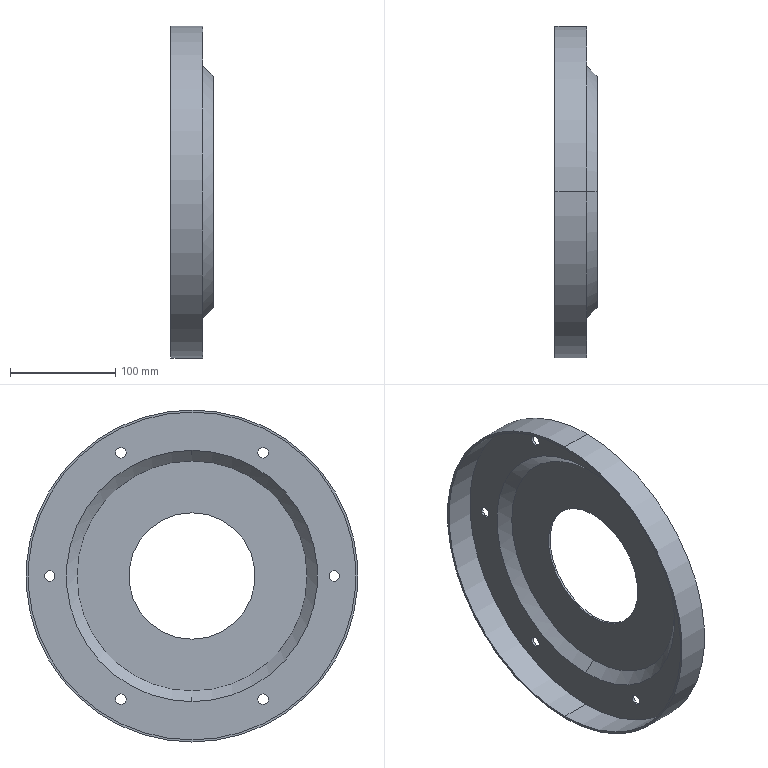Part | SolidWorks | features ICE 2, Revolution 1, Shell 1 | 1 solid | 27 faces | box 40 x 315 x 315 mm | volume 193331 mm3 | cylinder 18 | plane 5 | cone 4 | commonest cylinder face diameters 10 x12 120 x2 311 x2 315 x2
STEP:
#1=CARTESIAN_POINT('',(28.,135.,-5.));
#2=VERTEX_POINT('',#1);
#3=CARTESIAN_POINT('',(28.,135.,5.));
#4=VERTEX_POINT('',#3);
#5=CARTESIAN_POINT('',(28.,135.,0.));
#6=DIRECTION('',(-1.,0.,0.));
#7=DIRECTION('',(0.,0.,1.));
#8=AXIS2_PLACEMENT_3D('',#5,#6,#7);
#9=CIRCLE('',#8,5.);
#10=EDGE_CURVE('',#2,#4,#9,.T.);
#11=ORIENTED_EDGE('',*,*,#10,.T.);
#12=CARTESIAN_POINT('',(30.,135.,5.));
#13=VERTEX_POINT('',#12);
#14=CARTESIAN_POINT('',(-20.,135.,5.));
#15=DIRECTION('',(1.,0.,0.));
#16=VECTOR('',#15,1000.);
#17=LINE('',#14,#16);
#18=EDGE_CURVE('',#4,#13,#17,.T.);
#19=ORIENTED_EDGE('',*,*,#18,.T.);
#20=CARTESIAN_POINT('',(30.,135.,-5.));
#21=VERTEX_POINT('',#20);
#22=CARTESIAN_POINT('',(30.,135.,0.));
#23=DIRECTION('',(1.,0.,0.));
#24=DIRECTION('',(0.,0.,-1.));
#25=AXIS2_PLACEMENT_3D('',#22,#23,#24);
#26=CIRCLE('',#25,5.);
#27=EDGE_CURVE('',#13,#21,#26,.T.);
#28=ORIENTED_EDGE('',*,*,#27,.T.);
#29=CARTESIAN_POINT('',(-20.,135.,-5.));
#30=DIRECTION('',(1.,0.,0.));
#31=VECTOR('',#30,1000.);
#32=LINE('',#29,#31);
#33=EDGE_CURVE('',#2,#21,#32,.T.);
#34=ORIENTED_EDGE('',*,*,#33,.F.);
#35=EDGE_LOOP('',(#11,#19,#28,#34));
#36=FACE_OUTER_BOUND('',#35,.T.);
#37=CARTESIAN_POINT('',(-20.,135.,0.));
#38=DIRECTION('',(1.,0.,0.));
#39=DIRECTION('',(0.,0.,-1.));
#40=AXIS2_PLACEMENT_3D('',#37,#38,#39);
#41=CYLINDRICAL_SURFACE('',#40,5.);
#42=ADVANCED_FACE('',(#36),#41,.F.);
#43=CARTESIAN_POINT('',(28.,67.5,111.913));
#44=VERTEX_POINT('',#43);
#45=CARTESIAN_POINT('',(28.,67.5,121.913));
#46=VERTEX_POINT('',#45);
#47=CARTESIAN_POINT('',(28.,67.5,116.913));
#48=DIRECTION('',(-1.,0.,0.));
#49=DIRECTION('',(0.,0.,1.));
#50=AXIS2_PLACEMENT_3D('',#47,#48,#49);
#51=CIRCLE('',#50,5.);
#52=EDGE_CURVE('',#44,#46,#51,.T.);
#53=ORIENTED_EDGE('',*,*,#52,.T.);
#54=CARTESIAN_POINT('',(30.,67.5,121.913));
#55=VERTEX_POINT('',#54);
#56=CARTESIAN_POINT('',(-20.,67.5,121.913));
#57=DIRECTION('',(1.,0.,0.));
#58=VECTOR('',#57,1000.);
#59=LINE('',#56,#58);
#60=EDGE_CURVE('',#46,#55,#59,.T.);
#61=ORIENTED_EDGE('',*,*,#60,.T.);
#62=CARTESIAN_POINT('',(30.,67.5,111.913));
#63=VERTEX_POINT('',#62);
#64=CARTESIAN_POINT('',(30.,67.5,116.913));
#65=DIRECTION('',(1.,0.,0.));
#66=DIRECTION('',(0.,0.,-1.));
#67=AXIS2_PLACEMENT_3D('',#64,#65,#66);
#68=CIRCLE('',#67,5.);
#69=EDGE_CURVE('',#55,#63,#68,.T.);
#70=ORIENTED_EDGE('',*,*,#69,.T.);
#71=CARTESIAN_POINT('',(-20.,67.5,111.913));
#72=DIRECTION('',(1.,0.,0.));
#73=VECTOR('',#72,1000.);
#74=LINE('',#71,#73);
#75=EDGE_CURVE('',#44,#63,#74,.T.);
#76=ORIENTED_EDGE('',*,*,#75,.F.);
#77=EDGE_LOOP('',(#53,#61,#70,#76));
#78=FACE_OUTER_BOUND('',#77,.T.);
#79=CARTESIAN_POINT('',(-20.,67.5,116.913));
#80=DIRECTION('',(1.,0.,0.));
#81=DIRECTION('',(0.,0.,-1.));
#82=AXIS2_PLACEMENT_3D('',#79,#80,#81);
#83=CYLINDRICAL_SURFACE('',#82,5.);
#84=ADVANCED_FACE('',(#78),#83,.F.);
#85=CARTESIAN_POINT('',(28.,-67.5,111.913));
#86=VERTEX_POINT('',#85);
#87=CARTESIAN_POINT('',(28.,-67.5,121.913));
#88=VERTEX_POINT('',#87);
#89=CARTESIAN_POINT('',(28.,-67.5,116.913));
#90=DIRECTION('',(-1.,0.,0.));
#91=DIRECTION('',(0.,0.,1.));
#92=AXIS2_PLACEMENT_3D('',#89,#90,#91);
#93=CIRCLE('',#92,5.);
#94=EDGE_CURVE('',#86,#88,#93,.T.);
#95=ORIENTED_EDGE('',*,*,#94,.T.);
#96=CARTESIAN_POINT('',(30.,-67.5,121.913));
#97=VERTEX_POINT('',#96);
#98=CARTESIAN_POINT('',(-20.,-67.5,121.913));
#99=DIRECTION('',(1.,0.,0.));
#100=VECTOR('',#99,1000.);
#101=LINE('',#98,#100);
#102=EDGE_CURVE('',#88,#97,#101,.T.);
#103=ORIENTED_EDGE('',*,*,#102,.T.);
#104=CARTESIAN_POINT('',(30.,-67.5,111.913));
#105=VERTEX_POINT('',#104);
#106=CARTESIAN_POINT('',(30.,-67.5,116.913));
#107=DIRECTION('',(1.,0.,0.));
#108=DIRECTION('',(0.,0.,-1.));
#109=AXIS2_PLACEMENT_3D('',#106,#107,#108);
#110=CIRCLE('',#109,5.);
#111=EDGE_CURVE('',#97,#105,#110,.T.);
#112=ORIENTED_EDGE('',*,*,#111,.T.);
#113=CARTESIAN_POINT('',(-20.,-67.5,111.913));
#114=DIRECTION('',(1.,0.,0.));
#115=VECTOR('',#114,1000.);
#116=LINE('',#113,#115);
#117=EDGE_CURVE('',#86,#105,#116,.T.);
#118=ORIENTED_EDGE('',*,*,#117,.F.);
#119=EDGE_LOOP('',(#95,#103,#112,#118));
#120=FACE_OUTER_BOUND('',#119,.T.);
#121=CARTESIAN_POINT('',(-20.,-67.5,116.913));
#122=DIRECTION('',(1.,0.,0.));
#123=DIRECTION('',(0.,0.,-1.));
#124=AXIS2_PLACEMENT_3D('',#121,#122,#123);
#125=CYLINDRICAL_SURFACE('',#124,5.);
#126=ADVANCED_FACE('',(#120),#125,.F.);
#127=CARTESIAN_POINT('',(28.,-135.,-5.));
#128=VERTEX_POINT('',#127);
#129=CARTESIAN_POINT('',(28.,-135.,5.));
#130=VERTEX_POINT('',#129);
#131=CARTESIAN_POINT('',(28.,-135.,0.));
#132=DIRECTION('',(-1.,0.,0.));
#133=DIRECTION('',(0.,0.,1.));
#134=AXIS2_PLACEMENT_3D('',#131,#132,#133);
#135=CIRCLE('',#134,5.);
#136=EDGE_CURVE('',#128,#130,#135,.T.);
#137=ORIENTED_EDGE('',*,*,#136,.T.);
#138=CARTESIAN_POINT('',(30.,-135.,5.));
#139=VERTEX_POINT('',#138);
#140=CARTESIAN_POINT('',(-20.,-135.,5.));
#141=DIRECTION('',(1.,0.,0.));
#142=VECTOR('',#141,1000.);
#143=LINE('',#140,#142);
#144=EDGE_CURVE('',#130,#139,#143,.T.);
#145=ORIENTED_EDGE('',*,*,#144,.T.);
#146=CARTESIAN_POINT('',(30.,-135.,-5.));
#147=VERTEX_POINT('',#146);
#148=CARTESIAN_POINT('',(30.,-135.,0.));
#149=DIRECTION('',(1.,0.,0.));
#150=DIRECTION('',(0.,0.,-1.));
#151=AXIS2_PLACEMENT_3D('',#148,#149,#150);
#152=CIRCLE('',#151,5.);
#153=EDGE_CURVE('',#139,#147,#152,.T.);
#154=ORIENTED_EDGE('',*,*,#153,.T.);
#155=CARTESIAN_POINT('',(-20.,-135.,-5.));
#156=DIRECTION('',(1.,0.,0.));
#157=VECTOR('',#156,1000.);
#158=LINE('',#155,#157);
#159=EDGE_CURVE('',#128,#147,#158,.T.);
#160=ORIENTED_EDGE('',*,*,#159,.F.);
#161=EDGE_LOOP('',(#137,#145,#154,#160));
#162=FACE_OUTER_BOUND('',#161,.T.);
#163=CARTESIAN_POINT('',(-20.,-135.,0.));
#164=DIRECTION('',(1.,0.,0.));
#165=DIRECTION('',(0.,0.,-1.));
#166=AXIS2_PLACEMENT_3D('',#163,#164,#165);
#167=CYLINDRICAL_SURFACE('',#166,5.);
#168=ADVANCED_FACE('',(#162),#167,.F.);
#169=CARTESIAN_POINT('',(28.,-67.5,-121.913));
#170=VERTEX_POINT('',#169);
#171=CARTESIAN_POINT('',(28.,-67.5,-111.913));
#172=VERTEX_POINT('',#171);
#173=CARTESIAN_POINT('',(28.,-67.5,-116.913));
#174=DIRECTION('',(-1.,0.,0.));
#175=DIRECTION('',(0.,0.,1.));
#176=AXIS2_PLACEMENT_3D('',#173,#174,#175);
#177=CIRCLE('',#176,5.);
#178=EDGE_CURVE('',#170,#172,#177,.T.);
#179=ORIENTED_EDGE('',*,*,#178,.T.);
#180=CARTESIAN_POINT('',(30.,-67.5,-111.913));
#181=VERTEX_POINT('',#180);
#182=CARTESIAN_POINT('',(-20.,-67.5,-111.913));
#183=DIRECTION('',(1.,0.,0.));
#184=VECTOR('',#183,1000.);
#185=LINE('',#182,#184);
#186=EDGE_CURVE('',#172,#181,#185,.T.);
#187=ORIENTED_EDGE('',*,*,#186,.T.);
#188=CARTESIAN_POINT('',(30.,-67.5,-121.913));
#189=VERTEX_POINT('',#188);
#190=CARTESIAN_POINT('',(30.,-67.5,-116.913));
#191=DIRECTION('',(1.,0.,0.));
#192=DIRECTION('',(0.,0.,-1.));
#193=AXIS2_PLACEMENT_3D('',#190,#191,#192);
#194=CIRCLE('',#193,5.);
#195=EDGE_CURVE('',#181,#189,#194,.T.);
#196=ORIENTED_EDGE('',*,*,#195,.T.);
#197=CARTESIAN_POINT('',(-20.,-67.5,-121.913));
#198=DIRECTION('',(1.,0.,0.));
#199=VECTOR('',#198,1000.);
#200=LINE('',#197,#199);
#201=EDGE_CURVE('',#170,#189,#200,.T.);
#202=ORIENTED_EDGE('',*,*,#201,.F.);
#203=EDGE_LOOP('',(#179,#187,#196,#202));
#204=FACE_OUTER_BOUND('',#203,.T.);
#205=CARTESIAN_POINT('',(-20.,-67.5,-116.913));
#206=DIRECTION('',(1.,0.,0.));
#207=DIRECTION('',(0.,0.,-1.));
#208=AXIS2_PLACEMENT_3D('',#205,#206,#207);
#209=CYLINDRICAL_SURFACE('',#208,5.);
#210=ADVANCED_FACE('',(#204),#209,.F.);
#211=CARTESIAN_POINT('',(28.,67.5,-121.913));
#212=VERTEX_POINT('',#211);
#213=CARTESIAN_POINT('',(28.,67.5,-111.913));
#214=VERTEX_POINT('',#213);
#215=CARTESIAN_POINT('',(28.,67.5,-116.913));
#216=DIRECTION('',(-1.,0.,0.));
#217=DIRECTION('',(0.,0.,1.));
#218=AXIS2_PLACEMENT_3D('',#215,#216,#217);
#219=CIRCLE('',#218,5.);
#220=EDGE_CURVE('',#212,#214,#219,.T.);
#221=ORIENTED_EDGE('',*,*,#220,.T.);
#222=CARTESIAN_POINT('',(30.,67.5,-111.913));
#223=VERTEX_POINT('',#222);
#224=CARTESIAN_POINT('',(-20.,67.5,-111.913));
#225=DIRECTION('',(1.,0.,0.));
#226=VECTOR('',#225,1000.);
#227=LINE('',#224,#226);
#228=EDGE_CURVE('',#214,#223,#227,.T.);
#229=ORIENTED_EDGE('',*,*,#228,.T.);
#230=CARTESIAN_POINT('',(30.,67.5,-121.913));
#231=VERTEX_POINT('',#230);
#232=CARTESIAN_POINT('',(30.,67.5,-116.913));
#233=DIRECTION('',(1.,0.,0.));
#234=DIRECTION('',(0.,0.,-1.));
#235=AXIS2_PLACEMENT_3D('',#232,#233,#234);
#236=CIRCLE('',#235,5.);
#237=EDGE_CURVE('',#223,#231,#236,.T.);
#238=ORIENTED_EDGE('',*,*,#237,.T.);
#239=CARTESIAN_POINT('',(-20.,67.5,-121.913));
#240=DIRECTION('',(1.,0.,0.));
#241=VECTOR('',#240,1000.);
#242=LINE('',#239,#241);
#243=EDGE_CURVE('',#212,#231,#242,.T.);
#244=ORIENTED_EDGE('',*,*,#243,.F.);
#245=EDGE_LOOP('',(#221,#229,#238,#244));
#246=FACE_OUTER_BOUND('',#245,.T.);
#247=CARTESIAN_POINT('',(-20.,67.5,-116.913));
#248=DIRECTION('',(1.,0.,0.));
#249=DIRECTION('',(0.,0.,-1.));
#250=AXIS2_PLACEMENT_3D('',#247,#248,#249);
#251=CYLINDRICAL_SURFACE('',#250,5.);
#252=ADVANCED_FACE('',(#246),#251,.F.);
#253=CARTESIAN_POINT('',(38.,0.,-60.));
#254=VERTEX_POINT('',#253);
#255=CARTESIAN_POINT('',(38.,0.,60.));
#256=VERTEX_POINT('',#255);
#257=CARTESIAN_POINT('',(38.,0.,0.));
#258=DIRECTION('',(-1.,0.,0.));
#259=DIRECTION('',(0.,0.,1.));
#260=AXIS2_PLACEMENT_3D('',#257,#258,#259);
#261=CIRCLE('',#260,60.);
#262=EDGE_CURVE('',#254,#256,#261,.T.);
#263=ORIENTED_EDGE('',*,*,#262,.T.);
#264=CARTESIAN_POINT('',(40.,0.,60.));
#265=VERTEX_POINT('',#264);
#266=CARTESIAN_POINT('',(-10.,0.,60.));
#267=DIRECTION('',(1.,0.,0.));
#268=VECTOR('',#267,1000.);
#269=LINE('',#266,#268);
#270=EDGE_CURVE('',#256,#265,#269,.T.);
#271=ORIENTED_EDGE('',*,*,#270,.T.);
#272=CARTESIAN_POINT('',(40.,0.,-60.));
#273=VERTEX_POINT('',#272);
#274=CARTESIAN_POINT('',(40.,0.,0.));
#275=DIRECTION('',(1.,0.,0.));
#276=DIRECTION('',(0.,0.,-1.));
#277=AXIS2_PLACEMENT_3D('',#274,#275,#276);
#278=CIRCLE('',#277,60.);
#279=EDGE_CURVE('',#265,#273,#278,.T.);
#280=ORIENTED_EDGE('',*,*,#279,.T.);
#281=CARTESIAN_POINT('',(-10.,0.,-60.));
#282=DIRECTION('',(1.,0.,0.));
#283=VECTOR('',#282,1000.);
#284=LINE('',#281,#283);
#285=EDGE_CURVE('',#254,#273,#284,.T.);
#286=ORIENTED_EDGE('',*,*,#285,.F.);
#287=EDGE_LOOP('',(#263,#271,#280,#286));
#288=FACE_OUTER_BOUND('',#287,.T.);
#289=CARTESIAN_POINT('',(-10.,0.,0.));
#290=DIRECTION('',(1.,0.,0.));
#291=DIRECTION('',(0.,0.,-1.));
#292=AXIS2_PLACEMENT_3D('',#289,#290,#291);
#293=CYLINDRICAL_SURFACE('',#292,60.);
#294=ADVANCED_FACE('',(#288),#293,.F.);
#295=CARTESIAN_POINT('',(38.,0.,-109.172));
#296=VERTEX_POINT('',#295);
#297=CARTESIAN_POINT('',(38.,0.,109.172));
#298=VERTEX_POINT('',#297);
#299=CARTESIAN_POINT('',(38.,0.,0.));
#300=DIRECTION('',(-1.,0.,0.));
#301=DIRECTION('',(0.,0.,1.));
#302=AXIS2_PLACEMENT_3D('',#299,#300,#301);
#303=CIRCLE('',#302,109.172);
#304=EDGE_CURVE('',#296,#298,#303,.T.);
#305=ORIENTED_EDGE('',*,*,#304,.F.);
#306=CARTESIAN_POINT('',(28.,0.,-119.172));
#307=VERTEX_POINT('',#306);
#308=CARTESIAN_POINT('',(38.586,0.,-108.586));
#309=DIRECTION('',(-0.7071,0.,-0.7071));
#310=VECTOR('',#309,1000.);
#311=LINE('',#308,#310);
#312=EDGE_CURVE('',#296,#307,#311,.T.);
#313=ORIENTED_EDGE('',*,*,#312,.T.);
#314=CARTESIAN_POINT('',(28.,0.,119.172));
#315=VERTEX_POINT('',#314);
#316=CARTESIAN_POINT('',(28.,0.,0.));
#317=DIRECTION('',(-1.,0.,0.));
#318=DIRECTION('',(0.,0.,1.));
#319=AXIS2_PLACEMENT_3D('',#316,#317,#318);
#320=CIRCLE('',#319,119.172);
#321=EDGE_CURVE('',#307,#315,#320,.T.);
#322=ORIENTED_EDGE('',*,*,#321,.T.);
#323=CARTESIAN_POINT('',(38.586,0.,108.586));
#324=DIRECTION('',(-0.7071,0.,0.7071));
#325=VECTOR('',#324,1000.);
#326=LINE('',#323,#325);
#327=EDGE_CURVE('',#298,#315,#326,.T.);
#328=ORIENTED_EDGE('',*,*,#327,.F.);
#329=EDGE_LOOP('',(#305,#313,#322,#328));
#330=FACE_OUTER_BOUND('',#329,.T.);
#331=CARTESIAN_POINT('',(38.586,0.,0.));
#332=DIRECTION('',(-1.,0.,0.));
#333=DIRECTION('',(0.,0.,1.));
#334=AXIS2_PLACEMENT_3D('',#331,#332,#333);
#335=CONICAL_SURFACE('',#334,108.586,0.7854);
#336=ADVANCED_FACE('',(#330),#335,.F.);
#337=CARTESIAN_POINT('',(28.,0.,-155.5));
#338=VERTEX_POINT('',#337);
#339=CARTESIAN_POINT('',(28.,0.,155.5));
#340=VERTEX_POINT('',#339);
#341=CARTESIAN_POINT('',(28.,0.,0.));
#342=DIRECTION('',(-1.,0.,0.));
#343=DIRECTION('',(0.,0.,1.));
#344=AXIS2_PLACEMENT_3D('',#341,#342,#343);
#345=CIRCLE('',#344,155.5);
#346=EDGE_CURVE('',#338,#340,#345,.T.);
#347=ORIENTED_EDGE('',*,*,#346,.F.);
#348=CARTESIAN_POINT('',(0.,0.,-155.5));
#349=VERTEX_POINT('',#348);
#350=CARTESIAN_POINT('',(0.,0.,-155.5));
#351=DIRECTION('',(-1.,0.,0.));
#352=VECTOR('',#351,1000.);
#353=LINE('',#350,#352);
#354=EDGE_CURVE('',#338,#349,#353,.T.);
#355=ORIENTED_EDGE('',*,*,#354,.T.);
#356=CARTESIAN_POINT('',(0.,0.,155.5));
#357=VERTEX_POINT('',#356);
#358=CARTESIAN_POINT('',(0.,0.,0.));
#359=DIRECTION('',(-1.,0.,0.));
#360=DIRECTION('',(0.,0.,-1.));
#361=AXIS2_PLACEMENT_3D('',#358,#359,#360);
#362=CIRCLE('',#361,155.5);
#363=EDGE_CURVE('',#349,#357,#362,.T.);
#364=ORIENTED_EDGE('',*,*,#363,.T.);
#365=CARTESIAN_POINT('',(0.,0.,155.5));
#366=DIRECTION('',(-1.,0.,0.));
#367=VECTOR('',#366,1000.);
#368=LINE('',#365,#367);
#369=EDGE_CURVE('',#340,#357,#368,.T.);
#370=ORIENTED_EDGE('',*,*,#369,.F.);
#371=EDGE_LOOP('',(#347,#355,#364,#370));
#372=FACE_OUTER_BOUND('',#371,.T.);
#373=CARTESIAN_POINT('',(0.,0.,0.));
#374=DIRECTION('',(-1.,0.,0.));
#375=DIRECTION('',(0.,0.,1.));
#376=AXIS2_PLACEMENT_3D('',#373,#374,#375);
#377=CYLINDRICAL_SURFACE('',#376,155.5);
#378=ADVANCED_FACE('',(#372),#377,.F.);
#379=CARTESIAN_POINT('',(40.,0.,110.));
#380=VERTEX_POINT('',#379);
#381=CARTESIAN_POINT('',(40.,0.,-110.));
#382=VERTEX_POINT('',#381);
#383=CARTESIAN_POINT('',(40.,0.,0.));
#384=DIRECTION('',(-1.,0.,0.));
#385=DIRECTION('',(0.,0.,1.));
#386=AXIS2_PLACEMENT_3D('',#383,#384,#385);
#387=CIRCLE('',#386,110.);
#388=EDGE_CURVE('',#380,#382,#387,.T.);
#389=ORIENTED_EDGE('',*,*,#388,.T.);
#390=CARTESIAN_POINT('',(30.,0.,-120.));
#391=VERTEX_POINT('',#390);
#392=CARTESIAN_POINT('',(40.,0.,-110.));
#393=DIRECTION('',(-0.7071,0.,-0.7071));
#394=VECTOR('',#393,1000.);
#395=LINE('',#392,#394);
#396=EDGE_CURVE('',#382,#391,#395,.T.);
#397=ORIENTED_EDGE('',*,*,#396,.T.);
#398=CARTESIAN_POINT('',(30.,0.,120.));
#399=VERTEX_POINT('',#398);
#400=CARTESIAN_POINT('',(30.,0.,0.));
#401=DIRECTION('',(-1.,0.,0.));
#402=DIRECTION('',(0.,0.,1.));
#403=AXIS2_PLACEMENT_3D('',#400,#401,#402);
#404=CIRCLE('',#403,120.);
#405=EDGE_CURVE('',#399,#391,#404,.T.);
#406=ORIENTED_EDGE('',*,*,#405,.F.);
#407=CARTESIAN_POINT('',(40.,0.,110.));
#408=DIRECTION('',(-0.7071,0.,0.7071));
#409=VECTOR('',#408,1000.);
#410=LINE('',#407,#409);
#411=EDGE_CURVE('',#380,#399,#410,.T.);
#412=ORIENTED_EDGE('',*,*,#411,.F.);
#413=EDGE_LOOP('',(#389,#397,#406,#412));
#414=FACE_OUTER_BOUND('',#413,.T.);
#415=CARTESIAN_POINT('',(40.,0.,0.));
#416=DIRECTION('',(-1.,0.,0.));
#417=DIRECTION('',(0.,0.,1.));
#418=AXIS2_PLACEMENT_3D('',#415,#416,#417);
#419=CONICAL_SURFACE('',#418,110.,0.7854);
#420=ADVANCED_FACE('',(#414),#419,.T.);
#421=CARTESIAN_POINT('',(30.,0.,157.5));
#422=VERTEX_POINT('',#421);
#423=CARTESIAN_POINT('',(30.,0.,-157.5));
#424=VERTEX_POINT('',#423);
#425=CARTESIAN_POINT('',(30.,0.,0.));
#426=DIRECTION('',(-1.,0.,0.));
#427=DIRECTION('',(0.,0.,1.));
#428=AXIS2_PLACEMENT_3D('',#425,#426,#427);
#429=CIRCLE('',#428,157.5);
#430=EDGE_CURVE('',#422,#424,#429,.T.);
#431=ORIENTED_EDGE('',*,*,#430,.T.);
#432=CARTESIAN_POINT('',(0.,0.,-157.5));
#433=VERTEX_POINT('',#432);
#434=CARTESIAN_POINT('',(0.,0.,-157.5));
#435=DIRECTION('',(-1.,0.,0.));
#436=VECTOR('',#435,1000.);
#437=LINE('',#434,#436);
#438=EDGE_CURVE('',#424,#433,#437,.T.);
#439=ORIENTED_EDGE('',*,*,#438,.T.);
#440=CARTESIAN_POINT('',(0.,0.,157.5));
#441=VERTEX_POINT('',#440);
#442=CARTESIAN_POINT('',(0.,0.,0.));
#443=DIRECTION('',(-1.,0.,0.));
#444=DIRECTION('',(0.,0.,1.));
#445=AXIS2_PLACEMENT_3D('',#442,#443,#444);
#446=CIRCLE('',#445,157.5);
#447=EDGE_CURVE('',#441,#433,#446,.T.);
#448=ORIENTED_EDGE('',*,*,#447,.F.);
#449=CARTESIAN_POINT('',(0.,0.,157.5));
#450=DIRECTION('',(-1.,0.,0.));
#451=VECTOR('',#450,1000.);
#452=LINE('',#449,#451);
#453=EDGE_CURVE('',#422,#441,#452,.T.);
#454=ORIENTED_EDGE('',*,*,#453,.F.);
#455=EDGE_LOOP('',(#431,#439,#448,#454));
#456=FACE_OUTER_BOUND('',#455,.T.);
#457=CARTESIAN_POINT('',(0.,0.,0.));
#458=DIRECTION('',(-1.,0.,0.));
#459=DIRECTION('',(0.,0.,1.));
#460=AXIS2_PLACEMENT_3D('',#457,#458,#459);
#461=CYLINDRICAL_SURFACE('',#460,157.5);
#462=ADVANCED_FACE('',(#456),#461,.T.);
#463=CARTESIAN_POINT('',(0.,0.,0.));
#464=DIRECTION('',(-1.,0.,0.));
#465=DIRECTION('',(0.,0.,-1.));
#466=AXIS2_PLACEMENT_3D('',#463,#464,#465);
#467=CIRCLE('',#466,155.5);
#468=EDGE_CURVE('',#357,#349,#467,.T.);
#469=ORIENTED_EDGE('',*,*,#468,.F.);
#470=ORIENTED_EDGE('',*,*,#363,.F.);
#471=EDGE_LOOP('',(#469,#470));
#472=FACE_BOUND('',#471,.T.);
#473=ORIENTED_EDGE('',*,*,#447,.T.);
#474=CARTESIAN_POINT('',(0.,0.,0.));
#475=DIRECTION('',(-1.,0.,0.));
#476=DIRECTION('',(0.,0.,1.));
#477=AXIS2_PLACEMENT_3D('',#474,#475,#476);
#478=CIRCLE('',#477,157.5);
#479=EDGE_CURVE('',#433,#441,#478,.T.);
#480=ORIENTED_EDGE('',*,*,#479,.T.);
#481=EDGE_LOOP('',(#473,#480));
#482=FACE_OUTER_BOUND('',#481,.T.);
#483=CARTESIAN_POINT('',(0.,0.,0.));
#484=DIRECTION('',(1.,0.,0.));
#485=DIRECTION('',(0.,0.,-1.));
#486=AXIS2_PLACEMENT_3D('',#483,#484,#485);
#487=PLANE('',#486);
#488=ADVANCED_FACE('',(#472,#482),#487,.F.);
#489=ORIENTED_EDGE('',*,*,#438,.F.);
#490=CARTESIAN_POINT('',(30.,0.,0.));
#491=DIRECTION('',(-1.,0.,0.));
#492=DIRECTION('',(0.,0.,1.));
#493=AXIS2_PLACEMENT_3D('',#490,#491,#492);
#494=CIRCLE('',#493,157.5);
#495=EDGE_CURVE('',#424,#422,#494,.T.);
#496=ORIENTED_EDGE('',*,*,#495,.T.);
#497=ORIENTED_EDGE('',*,*,#453,.T.);
#498=ORIENTED_EDGE('',*,*,#479,.F.);
#499=EDGE_LOOP('',(#489,#496,#497,#498));
#500=FACE_OUTER_BOUND('',#499,.T.);
#501=CARTESIAN_POINT('',(0.,0.,0.));
#502=DIRECTION('',(-1.,0.,0.));
#503=DIRECTION('',(0.,0.,1.));
#504=AXIS2_PLACEMENT_3D('',#501,#502,#503);
#505=CYLINDRICAL_SURFACE('',#504,157.5);
#506=ADVANCED_FACE('',(#500),#505,.T.);
#507=CARTESIAN_POINT('',(30.,135.,0.));
#508=DIRECTION('',(1.,0.,0.));
#509=DIRECTION('',(0.,0.,-1.));
#510=AXIS2_PLACEMENT_3D('',#507,#508,#509);
#511=CIRCLE('',#510,5.);
#512=EDGE_CURVE('',#21,#13,#511,.T.);
#513=ORIENTED_EDGE('',*,*,#512,.F.);
#514=ORIENTED_EDGE('',*,*,#27,.F.);
#515=EDGE_LOOP('',(#513,#514));
#516=FACE_BOUND('',#515,.T.);
#517=CARTESIAN_POINT('',(30.,67.5,116.913));
#518=DIRECTION('',(1.,0.,0.));
#519=DIRECTION('',(0.,0.,-1.));
#520=AXIS2_PLACEMENT_3D('',#517,#518,#519);
#521=CIRCLE('',#520,5.);
#522=EDGE_CURVE('',#63,#55,#521,.T.);
#523=ORIENTED_EDGE('',*,*,#522,.F.);
#524=ORIENTED_EDGE('',*,*,#69,.F.);
#525=EDGE_LOOP('',(#523,#524));
#526=FACE_BOUND('',#525,.T.);
#527=CARTESIAN_POINT('',(30.,-67.5,116.913));
#528=DIRECTION('',(1.,0.,0.));
#529=DIRECTION('',(0.,0.,-1.));
#530=AXIS2_PLACEMENT_3D('',#527,#528,#529);
#531=CIRCLE('',#530,5.);
#532=EDGE_CURVE('',#105,#97,#531,.T.);
#533=ORIENTED_EDGE('',*,*,#532,.F.);
#534=ORIENTED_EDGE('',*,*,#111,.F.);
#535=EDGE_LOOP('',(#533,#534));
#536=FACE_BOUND('',#535,.T.);
#537=CARTESIAN_POINT('',(30.,-135.,0.));
#538=DIRECTION('',(1.,0.,0.));
#539=DIRECTION('',(0.,0.,-1.));
#540=AXIS2_PLACEMENT_3D('',#537,#538,#539);
#541=CIRCLE('',#540,5.);
#542=EDGE_CURVE('',#147,#139,#541,.T.);
#543=ORIENTED_EDGE('',*,*,#542,.F.);
#544=ORIENTED_EDGE('',*,*,#153,.F.);
#545=EDGE_LOOP('',(#543,#544));
#546=FACE_BOUND('',#545,.T.);
#547=CARTESIAN_POINT('',(30.,-67.5,-116.913));
#548=DIRECTION('',(1.,0.,0.));
#549=DIRECTION('',(0.,0.,-1.));
#550=AXIS2_PLACEMENT_3D('',#547,#548,#549);
#551=CIRCLE('',#550,5.);
#552=EDGE_CURVE('',#189,#181,#551,.T.);
#553=ORIENTED_EDGE('',*,*,#552,.F.);
#554=ORIENTED_EDGE('',*,*,#195,.F.);
#555=EDGE_LOOP('',(#553,#554));
#556=FACE_BOUND('',#555,.T.);
#557=CARTESIAN_POINT('',(30.,67.5,-116.913));
#558=DIRECTION('',(1.,0.,0.));
#559=DIRECTION('',(0.,0.,-1.));
#560=AXIS2_PLACEMENT_3D('',#557,#558,#559);
#561=CIRCLE('',#560,5.);
#562=EDGE_CURVE('',#231,#223,#561,.T.);
#563=ORIENTED_EDGE('',*,*,#562,.F.);
#564=ORIENTED_EDGE('',*,*,#237,.F.);
#565=EDGE_LOOP('',(#563,#564));
#566=FACE_BOUND('',#565,.T.);
#567=ORIENTED_EDGE('',*,*,#430,.F.);
#568=ORIENTED_EDGE('',*,*,#495,.F.);
#569=EDGE_LOOP('',(#567,#568));
#570=FACE_OUTER_BOUND('',#569,.T.);
#571=ORIENTED_EDGE('',*,*,#405,.T.);
#572=CARTESIAN_POINT('',(30.,0.,0.));
#573=DIRECTION('',(-1.,0.,0.));
#574=DIRECTION('',(0.,0.,1.));
#575=AXIS2_PLACEMENT_3D('',#572,#573,#574);
#576=CIRCLE('',#575,120.);
#577=EDGE_CURVE('',#391,#399,#576,.T.);
#578=ORIENTED_EDGE('',*,*,#577,.T.);
#579=EDGE_LOOP('',(#571,#578));
#580=FACE_BOUND('',#579,.T.);
#581=CARTESIAN_POINT('',(30.,0.,-157.5));
#582=DIRECTION('',(-1.,0.,0.));
#583=DIRECTION('',(0.,0.,1.));
#584=AXIS2_PLACEMENT_3D('',#581,#582,#583);
#585=PLANE('',#584);
#586=ADVANCED_FACE('',(#516,#526,#536,#546,#556,#566,#570,#580),#585,.F.);
#587=ORIENTED_EDGE('',*,*,#396,.F.);
#588=CARTESIAN_POINT('',(40.,0.,0.));
#589=DIRECTION('',(-1.,0.,0.));
#590=DIRECTION('',(0.,0.,1.));
#591=AXIS2_PLACEMENT_3D('',#588,#589,#590);
#592=CIRCLE('',#591,110.);
#593=EDGE_CURVE('',#382,#380,#592,.T.);
#594=ORIENTED_EDGE('',*,*,#593,.T.);
#595=ORIENTED_EDGE('',*,*,#411,.T.);
#596=ORIENTED_EDGE('',*,*,#577,.F.);
#597=EDGE_LOOP('',(#587,#594,#595,#596));
#598=FACE_OUTER_BOUND('',#597,.T.);
#599=CARTESIAN_POINT('',(40.,0.,0.));
#600=DIRECTION('',(-1.,0.,0.));
#601=DIRECTION('',(0.,0.,1.));
#602=AXIS2_PLACEMENT_3D('',#599,#600,#601);
#603=CONICAL_SURFACE('',#602,110.,0.7854);
#604=ADVANCED_FACE('',(#598),#603,.T.);
#605=CARTESIAN_POINT('',(40.,0.,0.));
#606=DIRECTION('',(1.,0.,0.));
#607=DIRECTION('',(0.,0.,-1.));
#608=AXIS2_PLACEMENT_3D('',#605,#606,#607);
#609=CIRCLE('',#608,60.);
#610=EDGE_CURVE('',#273,#265,#609,.T.);
#611=ORIENTED_EDGE('',*,*,#610,.F.);
#612=ORIENTED_EDGE('',*,*,#279,.F.);
#613=EDGE_LOOP('',(#611,#612));
#614=FACE_BOUND('',#613,.T.);
#615=ORIENTED_EDGE('',*,*,#388,.F.);
#616=ORIENTED_EDGE('',*,*,#593,.F.);
#617=EDGE_LOOP('',(#615,#616));
#618=FACE_OUTER_BOUND('',#617,.T.);
#619=CARTESIAN_POINT('',(40.,0.,-110.));
#620=DIRECTION('',(-1.,0.,0.));
#621=DIRECTION('',(0.,0.,1.));
#622=AXIS2_PLACEMENT_3D('',#619,#620,#621);
#623=PLANE('',#622);
#624=ADVANCED_FACE('',(#614,#618),#623,.F.);
#625=ORIENTED_EDGE('',*,*,#354,.F.);
#626=CARTESIAN_POINT('',(28.,0.,0.));
#627=DIRECTION('',(-1.,0.,0.));
#628=DIRECTION('',(0.,0.,1.));
#629=AXIS2_PLACEMENT_3D('',#626,#627,#628);
#630=CIRCLE('',#629,155.5);
#631=EDGE_CURVE('',#340,#338,#630,.T.);
#632=ORIENTED_EDGE('',*,*,#631,.F.);
#633=ORIENTED_EDGE('',*,*,#369,.T.);
#634=ORIENTED_EDGE('',*,*,#468,.T.);
#635=EDGE_LOOP('',(#625,#632,#633,#634));
#636=FACE_OUTER_BOUND('',#635,.T.);
#637=CARTESIAN_POINT('',(0.,0.,0.));
#638=DIRECTION('',(-1.,0.,0.));
#639=DIRECTION('',(0.,0.,1.));
#640=AXIS2_PLACEMENT_3D('',#637,#638,#639);
#641=CYLINDRICAL_SURFACE('',#640,155.5);
#642=ADVANCED_FACE('',(#636),#641,.F.);
#643=ORIENTED_EDGE('',*,*,#10,.F.);
#644=CARTESIAN_POINT('',(28.,135.,0.));
#645=DIRECTION('',(-1.,0.,0.));
#646=DIRECTION('',(0.,0.,1.));
#647=AXIS2_PLACEMENT_3D('',#644,#645,#646);
#648=CIRCLE('',#647,5.);
#649=EDGE_CURVE('',#4,#2,#648,.T.);
#650=ORIENTED_EDGE('',*,*,#649,.F.);
#651=EDGE_LOOP('',(#643,#650));
#652=FACE_BOUND('',#651,.T.);
#653=ORIENTED_EDGE('',*,*,#52,.F.);
#654=CARTESIAN_POINT('',(28.,67.5,116.913));
#655=DIRECTION('',(-1.,0.,0.));
#656=DIRECTION('',(0.,0.,1.));
#657=AXIS2_PLACEMENT_3D('',#654,#655,#656);
#658=CIRCLE('',#657,5.);
#659=EDGE_CURVE('',#46,#44,#658,.T.);
#660=ORIENTED_EDGE('',*,*,#659,.F.);
#661=EDGE_LOOP('',(#653,#660));
#662=FACE_BOUND('',#661,.T.);
#663=ORIENTED_EDGE('',*,*,#94,.F.);
#664=CARTESIAN_POINT('',(28.,-67.5,116.913));
#665=DIRECTION('',(-1.,0.,0.));
#666=DIRECTION('',(0.,0.,1.));
#667=AXIS2_PLACEMENT_3D('',#664,#665,#666);
#668=CIRCLE('',#667,5.);
#669=EDGE_CURVE('',#88,#86,#668,.T.);
#670=ORIENTED_EDGE('',*,*,#669,.F.);
#671=EDGE_LOOP('',(#663,#670));
#672=FACE_BOUND('',#671,.T.);
#673=ORIENTED_EDGE('',*,*,#136,.F.);
#674=CARTESIAN_POINT('',(28.,-135.,0.));
#675=DIRECTION('',(-1.,0.,0.));
#676=DIRECTION('',(0.,0.,1.));
#677=AXIS2_PLACEMENT_3D('',#674,#675,#676);
#678=CIRCLE('',#677,5.);
#679=EDGE_CURVE('',#130,#128,#678,.T.);
#680=ORIENTED_EDGE('',*,*,#679,.F.);
#681=EDGE_LOOP('',(#673,#680));
#682=FACE_BOUND('',#681,.T.);
#683=ORIENTED_EDGE('',*,*,#178,.F.);
#684=CARTESIAN_POINT('',(28.,-67.5,-116.913));
#685=DIRECTION('',(-1.,0.,0.));
#686=DIRECTION('',(0.,0.,1.));
#687=AXIS2_PLACEMENT_3D('',#684,#685,#686);
#688=CIRCLE('',#687,5.);
#689=EDGE_CURVE('',#172,#170,#688,.T.);
#690=ORIENTED_EDGE('',*,*,#689,.F.);
#691=EDGE_LOOP('',(#683,#690));
#692=FACE_BOUND('',#691,.T.);
#693=ORIENTED_EDGE('',*,*,#220,.F.);
#694=CARTESIAN_POINT('',(28.,67.5,-116.913));
#695=DIRECTION('',(-1.,0.,0.));
#696=DIRECTION('',(0.,0.,1.));
#697=AXIS2_PLACEMENT_3D('',#694,#695,#696);
#698=CIRCLE('',#697,5.);
#699=EDGE_CURVE('',#214,#212,#698,.T.);
#700=ORIENTED_EDGE('',*,*,#699,.F.);
#701=EDGE_LOOP('',(#693,#700));
#702=FACE_BOUND('',#701,.T.);
#703=ORIENTED_EDGE('',*,*,#631,.T.);
#704=ORIENTED_EDGE('',*,*,#346,.T.);
#705=EDGE_LOOP('',(#703,#704));
#706=FACE_OUTER_BOUND('',#705,.T.);
#707=CARTESIAN_POINT('',(28.,0.,0.));
#708=DIRECTION('',(-1.,0.,0.));
#709=DIRECTION('',(0.,0.,1.));
#710=AXIS2_PLACEMENT_3D('',#707,#708,#709);
#711=CIRCLE('',#710,119.172);
#712=EDGE_CURVE('',#315,#307,#711,.T.);
#713=ORIENTED_EDGE('',*,*,#712,.F.);
#714=ORIENTED_EDGE('',*,*,#321,.F.);
#715=EDGE_LOOP('',(#713,#714));
#716=FACE_BOUND('',#715,.T.);
#717=CARTESIAN_POINT('',(28.,0.,-157.5));
#718=DIRECTION('',(-1.,0.,0.));
#719=DIRECTION('',(0.,0.,1.));
#720=AXIS2_PLACEMENT_3D('',#717,#718,#719);
#721=PLANE('',#720);
#722=ADVANCED_FACE('',(#652,#662,#672,#682,#692,#702,#706,#716),#721,.T.);
#723=ORIENTED_EDGE('',*,*,#312,.F.);
#724=CARTESIAN_POINT('',(38.,0.,0.));
#725=DIRECTION('',(-1.,0.,0.));
#726=DIRECTION('',(0.,0.,1.));
#727=AXIS2_PLACEMENT_3D('',#724,#725,#726);
#728=CIRCLE('',#727,109.172);
#729=EDGE_CURVE('',#298,#296,#728,.T.);
#730=ORIENTED_EDGE('',*,*,#729,.F.);
#731=ORIENTED_EDGE('',*,*,#327,.T.);
#732=ORIENTED_EDGE('',*,*,#712,.T.);
#733=EDGE_LOOP('',(#723,#730,#731,#732));
#734=FACE_OUTER_BOUND('',#733,.T.);
#735=CARTESIAN_POINT('',(38.586,0.,0.));
#736=DIRECTION('',(-1.,0.,0.));
#737=DIRECTION('',(0.,0.,1.));
#738=AXIS2_PLACEMENT_3D('',#735,#736,#737);
#739=CONICAL_SURFACE('',#738,108.586,0.7854);
#740=ADVANCED_FACE('',(#734),#739,.F.);
#741=ORIENTED_EDGE('',*,*,#262,.F.);
#742=CARTESIAN_POINT('',(38.,0.,0.));
#743=DIRECTION('',(-1.,0.,0.));
#744=DIRECTION('',(0.,0.,1.));
#745=AXIS2_PLACEMENT_3D('',#742,#743,#744);
#746=CIRCLE('',#745,60.);
#747=EDGE_CURVE('',#256,#254,#746,.T.);
#748=ORIENTED_EDGE('',*,*,#747,.F.);
#749=EDGE_LOOP('',(#741,#748));
#750=FACE_BOUND('',#749,.T.);
#751=ORIENTED_EDGE('',*,*,#729,.T.);
#752=ORIENTED_EDGE('',*,*,#304,.T.);
#753=EDGE_LOOP('',(#751,#752));
#754=FACE_OUTER_BOUND('',#753,.T.);
#755=CARTESIAN_POINT('',(38.,0.,-110.));
#756=DIRECTION('',(-1.,0.,0.));
#757=DIRECTION('',(0.,0.,1.));
#758=AXIS2_PLACEMENT_3D('',#755,#756,#757);
#759=PLANE('',#758);
#760=ADVANCED_FACE('',(#750,#754),#759,.T.);
#761=ORIENTED_EDGE('',*,*,#270,.F.);
#762=ORIENTED_EDGE('',*,*,#747,.T.);
#763=ORIENTED_EDGE('',*,*,#285,.T.);
#764=ORIENTED_EDGE('',*,*,#610,.T.);
#765=EDGE_LOOP('',(#761,#762,#763,#764));
#766=FACE_OUTER_BOUND('',#765,.T.);
#767=CARTESIAN_POINT('',(-10.,0.,0.));
#768=DIRECTION('',(1.,0.,0.));
#769=DIRECTION('',(0.,0.,-1.));
#770=AXIS2_PLACEMENT_3D('',#767,#768,#769);
#771=CYLINDRICAL_SURFACE('',#770,60.);
#772=ADVANCED_FACE('',(#766),#771,.F.);
#773=ORIENTED_EDGE('',*,*,#228,.F.);
#774=ORIENTED_EDGE('',*,*,#699,.T.);
#775=ORIENTED_EDGE('',*,*,#243,.T.);
#776=ORIENTED_EDGE('',*,*,#562,.T.);
#777=EDGE_LOOP('',(#773,#774,#775,#776));
#778=FACE_OUTER_BOUND('',#777,.T.);
#779=CARTESIAN_POINT('',(-20.,67.5,-116.913));
#780=DIRECTION('',(1.,0.,0.));
#781=DIRECTION('',(0.,0.,-1.));
#782=AXIS2_PLACEMENT_3D('',#779,#780,#781);
#783=CYLINDRICAL_SURFACE('',#782,5.);
#784=ADVANCED_FACE('',(#778),#783,.F.);
#785=ORIENTED_EDGE('',*,*,#186,.F.);
#786=ORIENTED_EDGE('',*,*,#689,.T.);
#787=ORIENTED_EDGE('',*,*,#201,.T.);
#788=ORIENTED_EDGE('',*,*,#552,.T.);
#789=EDGE_LOOP('',(#785,#786,#787,#788));
#790=FACE_OUTER_BOUND('',#789,.T.);
#791=CARTESIAN_POINT('',(-20.,-67.5,-116.913));
#792=DIRECTION('',(1.,0.,0.));
#793=DIRECTION('',(0.,0.,-1.));
#794=AXIS2_PLACEMENT_3D('',#791,#792,#793);
#795=CYLINDRICAL_SURFACE('',#794,5.);
#796=ADVANCED_FACE('',(#790),#795,.F.);
#797=ORIENTED_EDGE('',*,*,#144,.F.);
#798=ORIENTED_EDGE('',*,*,#679,.T.);
#799=ORIENTED_EDGE('',*,*,#159,.T.);
#800=ORIENTED_EDGE('',*,*,#542,.T.);
#801=EDGE_LOOP('',(#797,#798,#799,#800));
#802=FACE_OUTER_BOUND('',#801,.T.);
#803=CARTESIAN_POINT('',(-20.,-135.,0.));
#804=DIRECTION('',(1.,0.,0.));
#805=DIRECTION('',(0.,0.,-1.));
#806=AXIS2_PLACEMENT_3D('',#803,#804,#805);
#807=CYLINDRICAL_SURFACE('',#806,5.);
#808=ADVANCED_FACE('',(#802),#807,.F.);
#809=ORIENTED_EDGE('',*,*,#102,.F.);
#810=ORIENTED_EDGE('',*,*,#669,.T.);
#811=ORIENTED_EDGE('',*,*,#117,.T.);
#812=ORIENTED_EDGE('',*,*,#532,.T.);
#813=EDGE_LOOP('',(#809,#810,#811,#812));
#814=FACE_OUTER_BOUND('',#813,.T.);
#815=CARTESIAN_POINT('',(-20.,-67.5,116.913));
#816=DIRECTION('',(1.,0.,0.));
#817=DIRECTION('',(0.,0.,-1.));
#818=AXIS2_PLACEMENT_3D('',#815,#816,#817);
#819=CYLINDRICAL_SURFACE('',#818,5.);
#820=ADVANCED_FACE('',(#814),#819,.F.);
#821=ORIENTED_EDGE('',*,*,#60,.F.);
#822=ORIENTED_EDGE('',*,*,#659,.T.);
#823=ORIENTED_EDGE('',*,*,#75,.T.);
#824=ORIENTED_EDGE('',*,*,#522,.T.);
#825=EDGE_LOOP('',(#821,#822,#823,#824));
#826=FACE_OUTER_BOUND('',#825,.T.);
#827=CARTESIAN_POINT('',(-20.,67.5,116.913));
#828=DIRECTION('',(1.,0.,0.));
#829=DIRECTION('',(0.,0.,-1.));
#830=AXIS2_PLACEMENT_3D('',#827,#828,#829);
#831=CYLINDRICAL_SURFACE('',#830,5.);
#832=ADVANCED_FACE('',(#826),#831,.F.);
#833=ORIENTED_EDGE('',*,*,#18,.F.);
#834=ORIENTED_EDGE('',*,*,#649,.T.);
#835=ORIENTED_EDGE('',*,*,#33,.T.);
#836=ORIENTED_EDGE('',*,*,#512,.T.);
#837=EDGE_LOOP('',(#833,#834,#835,#836));
#838=FACE_OUTER_BOUND('',#837,.T.);
#839=CARTESIAN_POINT('',(-20.,135.,0.));
#840=DIRECTION('',(1.,0.,0.));
#841=DIRECTION('',(0.,0.,-1.));
#842=AXIS2_PLACEMENT_3D('',#839,#840,#841);
#843=CYLINDRICAL_SURFACE('',#842,5.);
#844=ADVANCED_FACE('',(#838),#843,.F.);
#845=CLOSED_SHELL('',(#42,#84,#126,#168,#210,#252,#294,#336,#378,#420,#462,#488,#506,#586,#604,#624,#642,#722,#740,#760,#772,#784,#796,#808,#820,#832,#844));
#846=MANIFOLD_SOLID_BREP('',#845);
#847=CARTESIAN_POINT('',(0.,0.,0.));
#848=DIRECTION('',(0.,0.,1.));
#849=DIRECTION('',(1.,0.,0.));
#850=AXIS2_PLACEMENT_3D('',#847,#848,#849);
#851=(LENGTH_UNIT()NAMED_UNIT(*)SI_UNIT(.MILLI.,.METRE.));
#852=UNCERTAINTY_MEASURE_WITH_UNIT(LENGTH_MEASURE(0.00001),#851,'','');
#853=(NAMED_UNIT(*)PLANE_ANGLE_UNIT()SI_UNIT($,.RADIAN.));
#854=(NAMED_UNIT(*)SI_UNIT($,.STERADIAN.)SOLID_ANGLE_UNIT());
#855=(GEOMETRIC_REPRESENTATION_CONTEXT(3)GLOBAL_UNCERTAINTY_ASSIGNED_CONTEXT((#852))GLOBAL_UNIT_ASSIGNED_CONTEXT((#851,#853,#854))REPRESENTATION_CONTEXT('',''));
#856=ADVANCED_BREP_SHAPE_REPRESENTATION('',(#846,#850),#855);